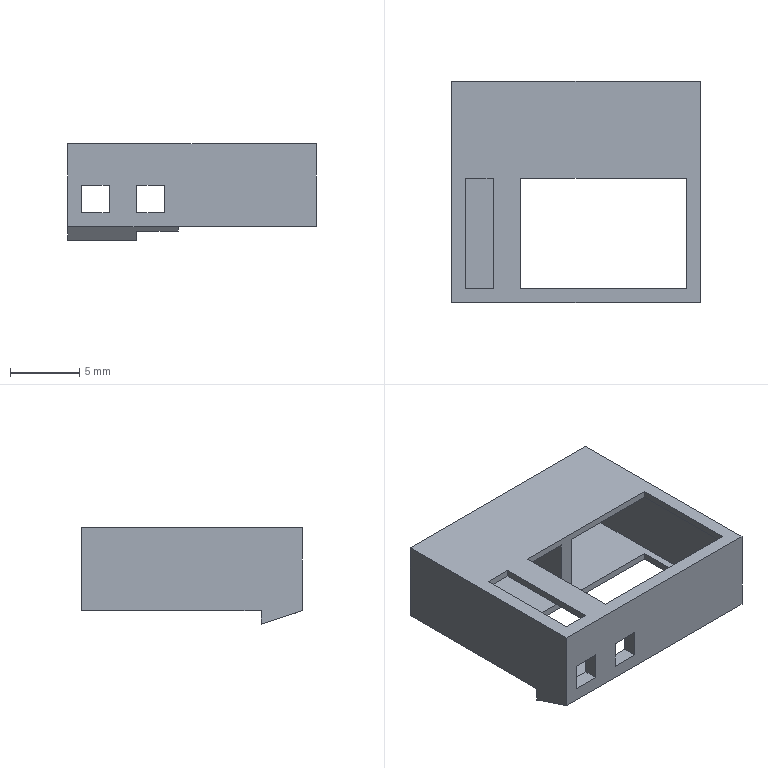Part | STEP file | 102000006983 | 1 solid | 34 faces | box 18 x 16 x 7 mm | volume 384 mm3 | plane 34
STEP:
#1=CARTESIAN_POINT('',(-9.,0.,0.));
#2=VERTEX_POINT('',#1);
#3=CARTESIAN_POINT('',(-9.,-13.,0.));
#4=VERTEX_POINT('',#3);
#5=CARTESIAN_POINT('',(-9.,-6.5,0.));
#6=DIRECTION('',(0.,-1.,0.));
#7=VECTOR('',#6,1.);
#8=LINE('',#5,#7);
#9=EDGE_CURVE('',#2,#4,#8,.T.);
#10=ORIENTED_EDGE('',*,*,#9,.T.);
#11=CARTESIAN_POINT('',(-9.,-13.,-1.));
#12=VERTEX_POINT('',#11);
#13=CARTESIAN_POINT('',(-9.,-13.,-0.5));
#14=DIRECTION('',(0.,0.,-1.));
#15=VECTOR('',#14,1.);
#16=LINE('',#13,#15);
#17=EDGE_CURVE('',#4,#12,#16,.T.);
#18=ORIENTED_EDGE('',*,*,#17,.T.);
#19=CARTESIAN_POINT('',(-9.,-16.,0.));
#20=VERTEX_POINT('',#19);
#21=CARTESIAN_POINT('',(-9.,-14.5,-0.5));
#22=DIRECTION('',(0.,-0.9487,0.3162));
#23=VECTOR('',#22,1.);
#24=LINE('',#21,#23);
#25=EDGE_CURVE('',#12,#20,#24,.T.);
#26=ORIENTED_EDGE('',*,*,#25,.T.);
#27=CARTESIAN_POINT('',(-9.,-16.,6.));
#28=VERTEX_POINT('',#27);
#29=CARTESIAN_POINT('',(-9.,-16.,3.));
#30=DIRECTION('',(0.,0.,-1.));
#31=VECTOR('',#30,1.);
#32=LINE('',#29,#31);
#33=EDGE_CURVE('',#28,#20,#32,.T.);
#34=ORIENTED_EDGE('',*,*,#33,.F.);
#35=CARTESIAN_POINT('',(-9.,0.,6.));
#36=VERTEX_POINT('',#35);
#37=CARTESIAN_POINT('',(-9.,-8.,6.));
#38=DIRECTION('',(0.,-1.,0.));
#39=VECTOR('',#38,1.);
#40=LINE('',#37,#39);
#41=EDGE_CURVE('',#36,#28,#40,.T.);
#42=ORIENTED_EDGE('',*,*,#41,.F.);
#43=CARTESIAN_POINT('',(-9.,0.,3.));
#44=DIRECTION('',(0.,0.,-1.));
#45=VECTOR('',#44,1.);
#46=LINE('',#43,#45);
#47=EDGE_CURVE('',#36,#2,#46,.T.);
#48=ORIENTED_EDGE('',*,*,#47,.T.);
#49=EDGE_LOOP('',(#10,#18,#26,#34,#42,#48));
#50=FACE_OUTER_BOUND('',#49,.T.);
#51=CARTESIAN_POINT('',(-9.,0.,6.));
#52=DIRECTION('',(1.,0.,0.));
#53=DIRECTION('',(0.,1.,0.));
#54=AXIS2_PLACEMENT_3D('',#51,#52,#53);
#55=PLANE('',#54);
#56=ADVANCED_FACE('',(#50),#55,.F.);
#57=CARTESIAN_POINT('',(-4.,-7.,0.));
#58=VERTEX_POINT('',#57);
#59=CARTESIAN_POINT('',(8.,-7.,0.));
#60=VERTEX_POINT('',#59);
#61=CARTESIAN_POINT('',(2.,-7.,0.));
#62=DIRECTION('',(1.,0.,0.));
#63=VECTOR('',#62,1.);
#64=LINE('',#61,#63);
#65=EDGE_CURVE('',#58,#60,#64,.T.);
#66=ORIENTED_EDGE('',*,*,#65,.F.);
#67=CARTESIAN_POINT('',(-4.,-13.,0.));
#68=VERTEX_POINT('',#67);
#69=CARTESIAN_POINT('',(-4.,-10.,0.));
#70=DIRECTION('',(0.,1.,0.));
#71=VECTOR('',#70,1.);
#72=LINE('',#69,#71);
#73=EDGE_CURVE('',#68,#58,#72,.T.);
#74=ORIENTED_EDGE('',*,*,#73,.F.);
#75=CARTESIAN_POINT('',(-6.5,-13.,0.));
#76=DIRECTION('',(-1.,0.,0.));
#77=VECTOR('',#76,1.);
#78=LINE('',#75,#77);
#79=EDGE_CURVE('',#68,#4,#78,.T.);
#80=ORIENTED_EDGE('',*,*,#79,.T.);
#81=ORIENTED_EDGE('',*,*,#9,.F.);
#82=CARTESIAN_POINT('',(9.,0.,0.));
#83=VERTEX_POINT('',#82);
#84=CARTESIAN_POINT('',(0.,0.,0.));
#85=DIRECTION('',(-1.,0.,0.));
#86=VECTOR('',#85,1.);
#87=LINE('',#84,#86);
#88=EDGE_CURVE('',#83,#2,#87,.T.);
#89=ORIENTED_EDGE('',*,*,#88,.F.);
#90=CARTESIAN_POINT('',(9.,-16.,0.));
#91=VERTEX_POINT('',#90);
#92=CARTESIAN_POINT('',(9.,-8.,0.));
#93=DIRECTION('',(0.,1.,0.));
#94=VECTOR('',#93,1.);
#95=LINE('',#92,#94);
#96=EDGE_CURVE('',#91,#83,#95,.T.);
#97=ORIENTED_EDGE('',*,*,#96,.F.);
#98=CARTESIAN_POINT('',(-1.,-16.,0.));
#99=VERTEX_POINT('',#98);
#100=CARTESIAN_POINT('',(4.,-16.,0.));
#101=DIRECTION('',(1.,0.,0.));
#102=VECTOR('',#101,1.);
#103=LINE('',#100,#102);
#104=EDGE_CURVE('',#99,#91,#103,.T.);
#105=ORIENTED_EDGE('',*,*,#104,.F.);
#106=CARTESIAN_POINT('',(-1.,-15.,0.));
#107=VERTEX_POINT('',#106);
#108=CARTESIAN_POINT('',(-1.,-15.5,0.));
#109=DIRECTION('',(0.,1.,0.));
#110=VECTOR('',#109,1.);
#111=LINE('',#108,#110);
#112=EDGE_CURVE('',#99,#107,#111,.T.);
#113=ORIENTED_EDGE('',*,*,#112,.T.);
#114=CARTESIAN_POINT('',(8.,-15.,0.));
#115=VERTEX_POINT('',#114);
#116=CARTESIAN_POINT('',(3.5,-15.,0.));
#117=DIRECTION('',(-1.,0.,0.));
#118=VECTOR('',#117,1.);
#119=LINE('',#116,#118);
#120=EDGE_CURVE('',#115,#107,#119,.T.);
#121=ORIENTED_EDGE('',*,*,#120,.F.);
#122=CARTESIAN_POINT('',(8.,-11.,0.));
#123=DIRECTION('',(0.,-1.,0.));
#124=VECTOR('',#123,1.);
#125=LINE('',#122,#124);
#126=EDGE_CURVE('',#60,#115,#125,.T.);
#127=ORIENTED_EDGE('',*,*,#126,.F.);
#128=EDGE_LOOP('',(#66,#74,#80,#81,#89,#97,#105,#113,#121,#127));
#129=FACE_OUTER_BOUND('',#128,.T.);
#130=CARTESIAN_POINT('',(0.,0.,0.));
#131=DIRECTION('',(0.,0.,1.));
#132=DIRECTION('',(1.,0.,0.));
#133=AXIS2_PLACEMENT_3D('',#130,#131,#132);
#134=PLANE('',#133);
#135=ADVANCED_FACE('',(#129),#134,.F.);
#136=CARTESIAN_POINT('',(-4.,-13.,-1.));
#137=VERTEX_POINT('',#136);
#138=CARTESIAN_POINT('',(-4.,-13.,-0.5));
#139=DIRECTION('',(0.,0.,-1.));
#140=VECTOR('',#139,1.);
#141=LINE('',#138,#140);
#142=EDGE_CURVE('',#68,#137,#141,.T.);
#143=ORIENTED_EDGE('',*,*,#142,.T.);
#144=CARTESIAN_POINT('',(-6.5,-13.,-1.));
#145=DIRECTION('',(-1.,0.,0.));
#146=VECTOR('',#145,1.);
#147=LINE('',#144,#146);
#148=EDGE_CURVE('',#137,#12,#147,.T.);
#149=ORIENTED_EDGE('',*,*,#148,.T.);
#150=ORIENTED_EDGE('',*,*,#17,.F.);
#151=ORIENTED_EDGE('',*,*,#79,.F.);
#152=EDGE_LOOP('',(#143,#149,#150,#151));
#153=FACE_OUTER_BOUND('',#152,.T.);
#154=CARTESIAN_POINT('',(-1.,-13.,-1.));
#155=DIRECTION('',(0.,1.,0.));
#156=DIRECTION('',(-1.,0.,0.));
#157=AXIS2_PLACEMENT_3D('',#154,#155,#156);
#158=PLANE('',#157);
#159=ADVANCED_FACE('',(#153),#158,.T.);
#160=CARTESIAN_POINT('',(-4.,-15.,-0.3333));
#161=VERTEX_POINT('',#160);
#162=CARTESIAN_POINT('',(-4.,-14.,-0.6667));
#163=DIRECTION('',(0.,-0.9487,0.3162));
#164=VECTOR('',#163,1.);
#165=LINE('',#162,#164);
#166=EDGE_CURVE('',#137,#161,#165,.T.);
#167=ORIENTED_EDGE('',*,*,#166,.T.);
#168=CARTESIAN_POINT('',(-1.,-15.,-0.3333));
#169=VERTEX_POINT('',#168);
#170=CARTESIAN_POINT('',(-2.5,-15.,-0.3333));
#171=DIRECTION('',(1.,0.,0.));
#172=VECTOR('',#171,1.);
#173=LINE('',#170,#172);
#174=EDGE_CURVE('',#161,#169,#173,.T.);
#175=ORIENTED_EDGE('',*,*,#174,.T.);
#176=CARTESIAN_POINT('',(-1.,-15.5,-0.1667));
#177=DIRECTION('',(0.,-0.9487,0.3162));
#178=VECTOR('',#177,1.);
#179=LINE('',#176,#178);
#180=EDGE_CURVE('',#169,#99,#179,.T.);
#181=ORIENTED_EDGE('',*,*,#180,.T.);
#182=CARTESIAN_POINT('',(-5.,-16.,0.));
#183=DIRECTION('',(1.,0.,0.));
#184=VECTOR('',#183,1.);
#185=LINE('',#182,#184);
#186=EDGE_CURVE('',#20,#99,#185,.T.);
#187=ORIENTED_EDGE('',*,*,#186,.F.);
#188=ORIENTED_EDGE('',*,*,#25,.F.);
#189=ORIENTED_EDGE('',*,*,#148,.F.);
#190=EDGE_LOOP('',(#167,#175,#181,#187,#188,#189));
#191=FACE_OUTER_BOUND('',#190,.T.);
#192=CARTESIAN_POINT('',(-1.,-16.,0.));
#193=DIRECTION('',(0.,-0.3162,-0.9487));
#194=DIRECTION('',(0.,0.9487,-0.3162));
#195=AXIS2_PLACEMENT_3D('',#192,#193,#194);
#196=PLANE('',#195);
#197=ADVANCED_FACE('',(#191),#196,.T.);
#198=ORIENTED_EDGE('',*,*,#186,.T.);
#199=ORIENTED_EDGE('',*,*,#104,.T.);
#200=CARTESIAN_POINT('',(9.,-16.,6.));
#201=VERTEX_POINT('',#200);
#202=CARTESIAN_POINT('',(9.,-16.,3.));
#203=DIRECTION('',(0.,0.,-1.));
#204=VECTOR('',#203,1.);
#205=LINE('',#202,#204);
#206=EDGE_CURVE('',#201,#91,#205,.T.);
#207=ORIENTED_EDGE('',*,*,#206,.F.);
#208=CARTESIAN_POINT('',(0.,-16.,6.));
#209=DIRECTION('',(1.,0.,0.));
#210=VECTOR('',#209,1.);
#211=LINE('',#208,#210);
#212=EDGE_CURVE('',#28,#201,#211,.T.);
#213=ORIENTED_EDGE('',*,*,#212,.F.);
#214=ORIENTED_EDGE('',*,*,#33,.T.);
#215=EDGE_LOOP('',(#198,#199,#207,#213,#214));
#216=FACE_OUTER_BOUND('',#215,.T.);
#217=CARTESIAN_POINT('',(-4.,-16.,1.));
#218=VERTEX_POINT('',#217);
#219=CARTESIAN_POINT('',(-2.,-16.,1.));
#220=VERTEX_POINT('',#219);
#221=CARTESIAN_POINT('',(-3.,-16.,1.));
#222=DIRECTION('',(1.,0.,0.));
#223=VECTOR('',#222,1.);
#224=LINE('',#221,#223);
#225=EDGE_CURVE('',#218,#220,#224,.T.);
#226=ORIENTED_EDGE('',*,*,#225,.F.);
#227=CARTESIAN_POINT('',(-4.,-16.,3.));
#228=VERTEX_POINT('',#227);
#229=CARTESIAN_POINT('',(-4.,-16.,2.));
#230=DIRECTION('',(0.,0.,-1.));
#231=VECTOR('',#230,1.);
#232=LINE('',#229,#231);
#233=EDGE_CURVE('',#228,#218,#232,.T.);
#234=ORIENTED_EDGE('',*,*,#233,.F.);
#235=CARTESIAN_POINT('',(-2.,-16.,3.));
#236=VERTEX_POINT('',#235);
#237=CARTESIAN_POINT('',(-3.,-16.,3.));
#238=DIRECTION('',(-1.,0.,0.));
#239=VECTOR('',#238,1.);
#240=LINE('',#237,#239);
#241=EDGE_CURVE('',#236,#228,#240,.T.);
#242=ORIENTED_EDGE('',*,*,#241,.F.);
#243=CARTESIAN_POINT('',(-2.,-16.,2.));
#244=DIRECTION('',(0.,0.,1.));
#245=VECTOR('',#244,1.);
#246=LINE('',#243,#245);
#247=EDGE_CURVE('',#220,#236,#246,.T.);
#248=ORIENTED_EDGE('',*,*,#247,.F.);
#249=EDGE_LOOP('',(#226,#234,#242,#248));
#250=FACE_BOUND('',#249,.T.);
#251=CARTESIAN_POINT('',(-8.,-16.,1.));
#252=VERTEX_POINT('',#251);
#253=CARTESIAN_POINT('',(-6.,-16.,1.));
#254=VERTEX_POINT('',#253);
#255=CARTESIAN_POINT('',(-7.,-16.,1.));
#256=DIRECTION('',(1.,0.,0.));
#257=VECTOR('',#256,1.);
#258=LINE('',#255,#257);
#259=EDGE_CURVE('',#252,#254,#258,.T.);
#260=ORIENTED_EDGE('',*,*,#259,.F.);
#261=CARTESIAN_POINT('',(-8.,-16.,3.));
#262=VERTEX_POINT('',#261);
#263=CARTESIAN_POINT('',(-8.,-16.,2.));
#264=DIRECTION('',(0.,0.,-1.));
#265=VECTOR('',#264,1.);
#266=LINE('',#263,#265);
#267=EDGE_CURVE('',#262,#252,#266,.T.);
#268=ORIENTED_EDGE('',*,*,#267,.F.);
#269=CARTESIAN_POINT('',(-6.,-16.,3.));
#270=VERTEX_POINT('',#269);
#271=CARTESIAN_POINT('',(-7.,-16.,3.));
#272=DIRECTION('',(-1.,0.,0.));
#273=VECTOR('',#272,1.);
#274=LINE('',#271,#273);
#275=EDGE_CURVE('',#270,#262,#274,.T.);
#276=ORIENTED_EDGE('',*,*,#275,.F.);
#277=CARTESIAN_POINT('',(-6.,-16.,2.));
#278=DIRECTION('',(0.,0.,1.));
#279=VECTOR('',#278,1.);
#280=LINE('',#277,#279);
#281=EDGE_CURVE('',#254,#270,#280,.T.);
#282=ORIENTED_EDGE('',*,*,#281,.F.);
#283=EDGE_LOOP('',(#260,#268,#276,#282));
#284=FACE_BOUND('',#283,.T.);
#285=CARTESIAN_POINT('',(-9.,-16.,6.));
#286=DIRECTION('',(0.,1.,0.));
#287=DIRECTION('',(0.,0.,1.));
#288=AXIS2_PLACEMENT_3D('',#285,#286,#287);
#289=PLANE('',#288);
#290=ADVANCED_FACE('',(#216,#250,#284),#289,.F.);
#291=ORIENTED_EDGE('',*,*,#41,.T.);
#292=ORIENTED_EDGE('',*,*,#212,.T.);
#293=CARTESIAN_POINT('',(9.,0.,6.));
#294=VERTEX_POINT('',#293);
#295=CARTESIAN_POINT('',(9.,-8.,6.));
#296=DIRECTION('',(0.,1.,0.));
#297=VECTOR('',#296,1.);
#298=LINE('',#295,#297);
#299=EDGE_CURVE('',#201,#294,#298,.T.);
#300=ORIENTED_EDGE('',*,*,#299,.T.);
#301=CARTESIAN_POINT('',(0.,0.,6.));
#302=DIRECTION('',(-1.,0.,0.));
#303=VECTOR('',#302,1.);
#304=LINE('',#301,#303);
#305=EDGE_CURVE('',#294,#36,#304,.T.);
#306=ORIENTED_EDGE('',*,*,#305,.T.);
#307=EDGE_LOOP('',(#291,#292,#300,#306));
#308=FACE_OUTER_BOUND('',#307,.T.);
#309=CARTESIAN_POINT('',(-4.,-7.,6.));
#310=VERTEX_POINT('',#309);
#311=CARTESIAN_POINT('',(-4.,-15.,6.));
#312=VERTEX_POINT('',#311);
#313=CARTESIAN_POINT('',(-4.,-11.,6.));
#314=DIRECTION('',(0.,-1.,0.));
#315=VECTOR('',#314,1.);
#316=LINE('',#313,#315);
#317=EDGE_CURVE('',#310,#312,#316,.T.);
#318=ORIENTED_EDGE('',*,*,#317,.F.);
#319=CARTESIAN_POINT('',(8.,-7.,6.));
#320=VERTEX_POINT('',#319);
#321=CARTESIAN_POINT('',(2.,-7.,6.));
#322=DIRECTION('',(-1.,0.,0.));
#323=VECTOR('',#322,1.);
#324=LINE('',#321,#323);
#325=EDGE_CURVE('',#320,#310,#324,.T.);
#326=ORIENTED_EDGE('',*,*,#325,.F.);
#327=CARTESIAN_POINT('',(8.,-15.,6.));
#328=VERTEX_POINT('',#327);
#329=CARTESIAN_POINT('',(8.,-11.,6.));
#330=DIRECTION('',(0.,1.,0.));
#331=VECTOR('',#330,1.);
#332=LINE('',#329,#331);
#333=EDGE_CURVE('',#328,#320,#332,.T.);
#334=ORIENTED_EDGE('',*,*,#333,.F.);
#335=CARTESIAN_POINT('',(2.,-15.,6.));
#336=DIRECTION('',(1.,0.,0.));
#337=VECTOR('',#336,1.);
#338=LINE('',#335,#337);
#339=EDGE_CURVE('',#312,#328,#338,.T.);
#340=ORIENTED_EDGE('',*,*,#339,.F.);
#341=EDGE_LOOP('',(#318,#326,#334,#340));
#342=FACE_BOUND('',#341,.T.);
#343=CARTESIAN_POINT('',(-8.,-7.,6.));
#344=VERTEX_POINT('',#343);
#345=CARTESIAN_POINT('',(-8.,-15.,6.));
#346=VERTEX_POINT('',#345);
#347=CARTESIAN_POINT('',(-8.,-11.,6.));
#348=DIRECTION('',(0.,-1.,0.));
#349=VECTOR('',#348,1.);
#350=LINE('',#347,#349);
#351=EDGE_CURVE('',#344,#346,#350,.T.);
#352=ORIENTED_EDGE('',*,*,#351,.F.);
#353=CARTESIAN_POINT('',(-6.,-7.,6.));
#354=VERTEX_POINT('',#353);
#355=CARTESIAN_POINT('',(-7.,-7.,6.));
#356=DIRECTION('',(-1.,0.,0.));
#357=VECTOR('',#356,1.);
#358=LINE('',#355,#357);
#359=EDGE_CURVE('',#354,#344,#358,.T.);
#360=ORIENTED_EDGE('',*,*,#359,.F.);
#361=CARTESIAN_POINT('',(-6.,-15.,6.));
#362=VERTEX_POINT('',#361);
#363=CARTESIAN_POINT('',(-6.,-11.,6.));
#364=DIRECTION('',(0.,1.,0.));
#365=VECTOR('',#364,1.);
#366=LINE('',#363,#365);
#367=EDGE_CURVE('',#362,#354,#366,.T.);
#368=ORIENTED_EDGE('',*,*,#367,.F.);
#369=CARTESIAN_POINT('',(-7.,-15.,6.));
#370=DIRECTION('',(1.,0.,0.));
#371=VECTOR('',#370,1.);
#372=LINE('',#369,#371);
#373=EDGE_CURVE('',#346,#362,#372,.T.);
#374=ORIENTED_EDGE('',*,*,#373,.F.);
#375=EDGE_LOOP('',(#352,#360,#368,#374));
#376=FACE_BOUND('',#375,.T.);
#377=CARTESIAN_POINT('',(0.,0.,6.));
#378=DIRECTION('',(0.,0.,1.));
#379=DIRECTION('',(1.,0.,0.));
#380=AXIS2_PLACEMENT_3D('',#377,#378,#379);
#381=PLANE('',#380);
#382=ADVANCED_FACE('',(#308,#342,#376),#381,.T.);
#383=ORIENTED_EDGE('',*,*,#88,.T.);
#384=ORIENTED_EDGE('',*,*,#47,.F.);
#385=ORIENTED_EDGE('',*,*,#305,.F.);
#386=CARTESIAN_POINT('',(9.,0.,3.));
#387=DIRECTION('',(0.,0.,-1.));
#388=VECTOR('',#387,1.);
#389=LINE('',#386,#388);
#390=EDGE_CURVE('',#294,#83,#389,.T.);
#391=ORIENTED_EDGE('',*,*,#390,.T.);
#392=EDGE_LOOP('',(#383,#384,#385,#391));
#393=FACE_OUTER_BOUND('',#392,.T.);
#394=CARTESIAN_POINT('',(0.5,0.,5.5));
#395=VERTEX_POINT('',#394);
#396=CARTESIAN_POINT('',(8.5,0.,5.5));
#397=VERTEX_POINT('',#396);
#398=CARTESIAN_POINT('',(4.5,0.,5.5));
#399=DIRECTION('',(1.,0.,0.));
#400=VECTOR('',#399,1.);
#401=LINE('',#398,#400);
#402=EDGE_CURVE('',#395,#397,#401,.T.);
#403=ORIENTED_EDGE('',*,*,#402,.F.);
#404=CARTESIAN_POINT('',(0.5,0.,0.5));
#405=VERTEX_POINT('',#404);
#406=CARTESIAN_POINT('',(0.5,0.,3.));
#407=DIRECTION('',(0.,0.,1.));
#408=VECTOR('',#407,1.);
#409=LINE('',#406,#408);
#410=EDGE_CURVE('',#405,#395,#409,.T.);
#411=ORIENTED_EDGE('',*,*,#410,.F.);
#412=CARTESIAN_POINT('',(8.5,0.,0.5));
#413=VERTEX_POINT('',#412);
#414=CARTESIAN_POINT('',(4.5,0.,0.5));
#415=DIRECTION('',(-1.,0.,0.));
#416=VECTOR('',#415,1.);
#417=LINE('',#414,#416);
#418=EDGE_CURVE('',#413,#405,#417,.T.);
#419=ORIENTED_EDGE('',*,*,#418,.F.);
#420=CARTESIAN_POINT('',(8.5,0.,3.));
#421=DIRECTION('',(0.,0.,-1.));
#422=VECTOR('',#421,1.);
#423=LINE('',#420,#422);
#424=EDGE_CURVE('',#397,#413,#423,.T.);
#425=ORIENTED_EDGE('',*,*,#424,.F.);
#426=EDGE_LOOP('',(#403,#411,#419,#425));
#427=FACE_BOUND('',#426,.T.);
#428=CARTESIAN_POINT('',(-8.5,0.,5.5));
#429=VERTEX_POINT('',#428);
#430=CARTESIAN_POINT('',(-0.5,0.,5.5));
#431=VERTEX_POINT('',#430);
#432=CARTESIAN_POINT('',(-4.5,0.,5.5));
#433=DIRECTION('',(1.,0.,0.));
#434=VECTOR('',#433,1.);
#435=LINE('',#432,#434);
#436=EDGE_CURVE('',#429,#431,#435,.T.);
#437=ORIENTED_EDGE('',*,*,#436,.F.);
#438=CARTESIAN_POINT('',(-8.5,0.,0.5));
#439=VERTEX_POINT('',#438);
#440=CARTESIAN_POINT('',(-8.5,0.,3.));
#441=DIRECTION('',(0.,0.,1.));
#442=VECTOR('',#441,1.);
#443=LINE('',#440,#442);
#444=EDGE_CURVE('',#439,#429,#443,.T.);
#445=ORIENTED_EDGE('',*,*,#444,.F.);
#446=CARTESIAN_POINT('',(-0.5,0.,0.5));
#447=VERTEX_POINT('',#446);
#448=CARTESIAN_POINT('',(-4.5,0.,0.5));
#449=DIRECTION('',(-1.,0.,0.));
#450=VECTOR('',#449,1.);
#451=LINE('',#448,#450);
#452=EDGE_CURVE('',#447,#439,#451,.T.);
#453=ORIENTED_EDGE('',*,*,#452,.F.);
#454=CARTESIAN_POINT('',(-0.5,0.,3.));
#455=DIRECTION('',(0.,0.,-1.));
#456=VECTOR('',#455,1.);
#457=LINE('',#454,#456);
#458=EDGE_CURVE('',#431,#447,#457,.T.);
#459=ORIENTED_EDGE('',*,*,#458,.F.);
#460=EDGE_LOOP('',(#437,#445,#453,#459));
#461=FACE_BOUND('',#460,.T.);
#462=CARTESIAN_POINT('',(-9.,0.,6.));
#463=DIRECTION('',(0.,-1.,0.));
#464=DIRECTION('',(0.,0.,-1.));
#465=AXIS2_PLACEMENT_3D('',#462,#463,#464);
#466=PLANE('',#465);
#467=ADVANCED_FACE('',(#393,#427,#461),#466,.F.);
#468=ORIENTED_EDGE('',*,*,#65,.T.);
#469=CARTESIAN_POINT('',(8.,-7.,0.5));
#470=VERTEX_POINT('',#469);
#471=CARTESIAN_POINT('',(8.,-7.,0.25));
#472=DIRECTION('',(0.,0.,1.));
#473=VECTOR('',#472,1.);
#474=LINE('',#471,#473);
#475=EDGE_CURVE('',#60,#470,#474,.T.);
#476=ORIENTED_EDGE('',*,*,#475,.T.);
#477=CARTESIAN_POINT('',(0.5,-7.,0.5));
#478=VERTEX_POINT('',#477);
#479=CARTESIAN_POINT('',(4.25,-7.,0.5));
#480=DIRECTION('',(-1.,0.,0.));
#481=VECTOR('',#480,1.);
#482=LINE('',#479,#481);
#483=EDGE_CURVE('',#470,#478,#482,.T.);
#484=ORIENTED_EDGE('',*,*,#483,.T.);
#485=CARTESIAN_POINT('',(0.5,-7.,5.5));
#486=VERTEX_POINT('',#485);
#487=CARTESIAN_POINT('',(0.5,-7.,3.));
#488=DIRECTION('',(0.,0.,1.));
#489=VECTOR('',#488,1.);
#490=LINE('',#487,#489);
#491=EDGE_CURVE('',#478,#486,#490,.T.);
#492=ORIENTED_EDGE('',*,*,#491,.T.);
#493=CARTESIAN_POINT('',(8.,-7.,5.5));
#494=VERTEX_POINT('',#493);
#495=CARTESIAN_POINT('',(4.25,-7.,5.5));
#496=DIRECTION('',(1.,0.,0.));
#497=VECTOR('',#496,1.);
#498=LINE('',#495,#497);
#499=EDGE_CURVE('',#486,#494,#498,.T.);
#500=ORIENTED_EDGE('',*,*,#499,.T.);
#501=CARTESIAN_POINT('',(8.,-7.,5.75));
#502=DIRECTION('',(0.,0.,1.));
#503=VECTOR('',#502,1.);
#504=LINE('',#501,#503);
#505=EDGE_CURVE('',#494,#320,#504,.T.);
#506=ORIENTED_EDGE('',*,*,#505,.T.);
#507=ORIENTED_EDGE('',*,*,#325,.T.);
#508=CARTESIAN_POINT('',(-4.,-7.,5.5));
#509=VERTEX_POINT('',#508);
#510=CARTESIAN_POINT('',(-4.,-7.,5.75));
#511=DIRECTION('',(0.,0.,1.));
#512=VECTOR('',#511,1.);
#513=LINE('',#510,#512);
#514=EDGE_CURVE('',#509,#310,#513,.T.);
#515=ORIENTED_EDGE('',*,*,#514,.F.);
#516=CARTESIAN_POINT('',(-0.5,-7.,5.5));
#517=VERTEX_POINT('',#516);
#518=CARTESIAN_POINT('',(-2.25,-7.,5.5));
#519=DIRECTION('',(1.,0.,0.));
#520=VECTOR('',#519,1.);
#521=LINE('',#518,#520);
#522=EDGE_CURVE('',#509,#517,#521,.T.);
#523=ORIENTED_EDGE('',*,*,#522,.T.);
#524=CARTESIAN_POINT('',(-0.5,-7.,0.5));
#525=VERTEX_POINT('',#524);
#526=CARTESIAN_POINT('',(-0.5,-7.,3.));
#527=DIRECTION('',(0.,0.,-1.));
#528=VECTOR('',#527,1.);
#529=LINE('',#526,#528);
#530=EDGE_CURVE('',#517,#525,#529,.T.);
#531=ORIENTED_EDGE('',*,*,#530,.T.);
#532=CARTESIAN_POINT('',(-4.,-7.,0.5));
#533=VERTEX_POINT('',#532);
#534=CARTESIAN_POINT('',(-2.25,-7.,0.5));
#535=DIRECTION('',(-1.,0.,0.));
#536=VECTOR('',#535,1.);
#537=LINE('',#534,#536);
#538=EDGE_CURVE('',#525,#533,#537,.T.);
#539=ORIENTED_EDGE('',*,*,#538,.T.);
#540=CARTESIAN_POINT('',(-4.,-7.,0.25));
#541=DIRECTION('',(0.,0.,1.));
#542=VECTOR('',#541,1.);
#543=LINE('',#540,#542);
#544=EDGE_CURVE('',#58,#533,#543,.T.);
#545=ORIENTED_EDGE('',*,*,#544,.F.);
#546=EDGE_LOOP('',(#468,#476,#484,#492,#500,#506,#507,#515,#523,#531,#539,#545));
#547=FACE_OUTER_BOUND('',#546,.T.);
#548=CARTESIAN_POINT('',(-4.,-7.,-1.001));
#549=DIRECTION('',(0.,1.,0.));
#550=DIRECTION('',(0.,0.,1.));
#551=AXIS2_PLACEMENT_3D('',#548,#549,#550);
#552=PLANE('',#551);
#553=ADVANCED_FACE('',(#547),#552,.F.);
#554=CARTESIAN_POINT('',(-4.,-15.,0.5));
#555=VERTEX_POINT('',#554);
#556=CARTESIAN_POINT('',(-4.,-11.,0.5));
#557=DIRECTION('',(0.,-1.,0.));
#558=VECTOR('',#557,1.);
#559=LINE('',#556,#558);
#560=EDGE_CURVE('',#533,#555,#559,.T.);
#561=ORIENTED_EDGE('',*,*,#560,.T.);
#562=CARTESIAN_POINT('',(-4.,-15.,0.08333));
#563=DIRECTION('',(0.,0.,1.));
#564=VECTOR('',#563,1.);
#565=LINE('',#562,#564);
#566=EDGE_CURVE('',#161,#555,#565,.T.);
#567=ORIENTED_EDGE('',*,*,#566,.F.);
#568=ORIENTED_EDGE('',*,*,#166,.F.);
#569=ORIENTED_EDGE('',*,*,#142,.F.);
#570=ORIENTED_EDGE('',*,*,#73,.T.);
#571=ORIENTED_EDGE('',*,*,#544,.T.);
#572=EDGE_LOOP('',(#561,#567,#568,#569,#570,#571));
#573=FACE_OUTER_BOUND('',#572,.T.);
#574=CARTESIAN_POINT('',(-4.,-7.,-1.001));
#575=DIRECTION('',(-1.,0.,0.));
#576=DIRECTION('',(0.,-1.,0.));
#577=AXIS2_PLACEMENT_3D('',#574,#575,#576);
#578=PLANE('',#577);
#579=ADVANCED_FACE('',(#573),#578,.F.);
#580=ORIENTED_EDGE('',*,*,#96,.T.);
#581=ORIENTED_EDGE('',*,*,#390,.F.);
#582=ORIENTED_EDGE('',*,*,#299,.F.);
#583=ORIENTED_EDGE('',*,*,#206,.T.);
#584=EDGE_LOOP('',(#580,#581,#582,#583));
#585=FACE_OUTER_BOUND('',#584,.T.);
#586=CARTESIAN_POINT('',(9.,0.,6.));
#587=DIRECTION('',(-1.,0.,0.));
#588=DIRECTION('',(0.,-1.,0.));
#589=AXIS2_PLACEMENT_3D('',#586,#587,#588);
#590=PLANE('',#589);
#591=ADVANCED_FACE('',(#585),#590,.F.);
#592=CARTESIAN_POINT('',(-1.,-15.,-0.1667));
#593=DIRECTION('',(0.,0.,1.));
#594=VECTOR('',#593,1.);
#595=LINE('',#592,#594);
#596=EDGE_CURVE('',#169,#107,#595,.T.);
#597=ORIENTED_EDGE('',*,*,#596,.T.);
#598=ORIENTED_EDGE('',*,*,#112,.F.);
#599=ORIENTED_EDGE('',*,*,#180,.F.);
#600=EDGE_LOOP('',(#597,#598,#599));
#601=FACE_OUTER_BOUND('',#600,.T.);
#602=CARTESIAN_POINT('',(-1.,0.,0.));
#603=DIRECTION('',(1.,0.,0.));
#604=DIRECTION('',(0.,0.,-1.));
#605=AXIS2_PLACEMENT_3D('',#602,#603,#604);
#606=PLANE('',#605);
#607=ADVANCED_FACE('',(#601),#606,.T.);
#608=ORIENTED_EDGE('',*,*,#566,.T.);
#609=CARTESIAN_POINT('',(-8.5,-15.,0.5));
#610=VERTEX_POINT('',#609);
#611=CARTESIAN_POINT('',(-6.25,-15.,0.5));
#612=DIRECTION('',(-1.,0.,0.));
#613=VECTOR('',#612,1.);
#614=LINE('',#611,#613);
#615=EDGE_CURVE('',#555,#610,#614,.T.);
#616=ORIENTED_EDGE('',*,*,#615,.T.);
#617=CARTESIAN_POINT('',(-8.5,-15.,5.5));
#618=VERTEX_POINT('',#617);
#619=CARTESIAN_POINT('',(-8.5,-15.,3.));
#620=DIRECTION('',(0.,0.,1.));
#621=VECTOR('',#620,1.);
#622=LINE('',#619,#621);
#623=EDGE_CURVE('',#610,#618,#622,.T.);
#624=ORIENTED_EDGE('',*,*,#623,.T.);
#625=CARTESIAN_POINT('',(-8.,-15.,5.5));
#626=VERTEX_POINT('',#625);
#627=CARTESIAN_POINT('',(-8.25,-15.,5.5));
#628=DIRECTION('',(1.,0.,0.));
#629=VECTOR('',#628,1.);
#630=LINE('',#627,#629);
#631=EDGE_CURVE('',#618,#626,#630,.T.);
#632=ORIENTED_EDGE('',*,*,#631,.T.);
#633=CARTESIAN_POINT('',(-8.,-15.,5.75));
#634=DIRECTION('',(0.,0.,1.));
#635=VECTOR('',#634,1.);
#636=LINE('',#633,#635);
#637=EDGE_CURVE('',#626,#346,#636,.T.);
#638=ORIENTED_EDGE('',*,*,#637,.T.);
#639=ORIENTED_EDGE('',*,*,#373,.T.);
#640=CARTESIAN_POINT('',(-6.,-15.,5.5));
#641=VERTEX_POINT('',#640);
#642=CARTESIAN_POINT('',(-6.,-15.,5.75));
#643=DIRECTION('',(0.,0.,1.));
#644=VECTOR('',#643,1.);
#645=LINE('',#642,#644);
#646=EDGE_CURVE('',#641,#362,#645,.T.);
#647=ORIENTED_EDGE('',*,*,#646,.F.);
#648=CARTESIAN_POINT('',(-4.,-15.,5.5));
#649=VERTEX_POINT('',#648);
#650=CARTESIAN_POINT('',(-5.,-15.,5.5));
#651=DIRECTION('',(1.,0.,0.));
#652=VECTOR('',#651,1.);
#653=LINE('',#650,#652);
#654=EDGE_CURVE('',#641,#649,#653,.T.);
#655=ORIENTED_EDGE('',*,*,#654,.T.);
#656=CARTESIAN_POINT('',(-4.,-15.,5.75));
#657=DIRECTION('',(0.,0.,1.));
#658=VECTOR('',#657,1.);
#659=LINE('',#656,#658);
#660=EDGE_CURVE('',#649,#312,#659,.T.);
#661=ORIENTED_EDGE('',*,*,#660,.T.);
#662=ORIENTED_EDGE('',*,*,#339,.T.);
#663=CARTESIAN_POINT('',(8.,-15.,5.5));
#664=VERTEX_POINT('',#663);
#665=CARTESIAN_POINT('',(8.,-15.,5.75));
#666=DIRECTION('',(0.,0.,1.));
#667=VECTOR('',#666,1.);
#668=LINE('',#665,#667);
#669=EDGE_CURVE('',#664,#328,#668,.T.);
#670=ORIENTED_EDGE('',*,*,#669,.F.);
#671=CARTESIAN_POINT('',(8.5,-15.,5.5));
#672=VERTEX_POINT('',#671);
#673=CARTESIAN_POINT('',(8.25,-15.,5.5));
#674=DIRECTION('',(1.,0.,0.));
#675=VECTOR('',#674,1.);
#676=LINE('',#673,#675);
#677=EDGE_CURVE('',#664,#672,#676,.T.);
#678=ORIENTED_EDGE('',*,*,#677,.T.);
#679=CARTESIAN_POINT('',(8.5,-15.,0.5));
#680=VERTEX_POINT('',#679);
#681=CARTESIAN_POINT('',(8.5,-15.,3.));
#682=DIRECTION('',(0.,0.,-1.));
#683=VECTOR('',#682,1.);
#684=LINE('',#681,#683);
#685=EDGE_CURVE('',#672,#680,#684,.T.);
#686=ORIENTED_EDGE('',*,*,#685,.T.);
#687=CARTESIAN_POINT('',(8.,-15.,0.5));
#688=VERTEX_POINT('',#687);
#689=CARTESIAN_POINT('',(8.25,-15.,0.5));
#690=DIRECTION('',(-1.,0.,0.));
#691=VECTOR('',#690,1.);
#692=LINE('',#689,#691);
#693=EDGE_CURVE('',#680,#688,#692,.T.);
#694=ORIENTED_EDGE('',*,*,#693,.T.);
#695=CARTESIAN_POINT('',(8.,-15.,0.25));
#696=DIRECTION('',(0.,0.,1.));
#697=VECTOR('',#696,1.);
#698=LINE('',#695,#697);
#699=EDGE_CURVE('',#115,#688,#698,.T.);
#700=ORIENTED_EDGE('',*,*,#699,.F.);
#701=ORIENTED_EDGE('',*,*,#120,.T.);
#702=ORIENTED_EDGE('',*,*,#596,.F.);
#703=ORIENTED_EDGE('',*,*,#174,.F.);
#704=EDGE_LOOP('',(#608,#616,#624,#632,#638,#639,#647,#655,#661,#662,#670,#678,#686,#694,#700,#701,#702,#703));
#705=FACE_OUTER_BOUND('',#704,.T.);
#706=CARTESIAN_POINT('',(-4.,-15.,1.));
#707=VERTEX_POINT('',#706);
#708=CARTESIAN_POINT('',(-4.,-15.,3.));
#709=VERTEX_POINT('',#708);
#710=CARTESIAN_POINT('',(-4.,-15.,2.));
#711=DIRECTION('',(0.,0.,1.));
#712=VECTOR('',#711,1.);
#713=LINE('',#710,#712);
#714=EDGE_CURVE('',#707,#709,#713,.T.);
#715=ORIENTED_EDGE('',*,*,#714,.F.);
#716=CARTESIAN_POINT('',(-2.,-15.,1.));
#717=VERTEX_POINT('',#716);
#718=CARTESIAN_POINT('',(-3.,-15.,1.));
#719=DIRECTION('',(-1.,0.,0.));
#720=VECTOR('',#719,1.);
#721=LINE('',#718,#720);
#722=EDGE_CURVE('',#717,#707,#721,.T.);
#723=ORIENTED_EDGE('',*,*,#722,.F.);
#724=CARTESIAN_POINT('',(-2.,-15.,3.));
#725=VERTEX_POINT('',#724);
#726=CARTESIAN_POINT('',(-2.,-15.,2.));
#727=DIRECTION('',(0.,0.,-1.));
#728=VECTOR('',#727,1.);
#729=LINE('',#726,#728);
#730=EDGE_CURVE('',#725,#717,#729,.T.);
#731=ORIENTED_EDGE('',*,*,#730,.F.);
#732=CARTESIAN_POINT('',(-3.,-15.,3.));
#733=DIRECTION('',(1.,0.,0.));
#734=VECTOR('',#733,1.);
#735=LINE('',#732,#734);
#736=EDGE_CURVE('',#709,#725,#735,.T.);
#737=ORIENTED_EDGE('',*,*,#736,.F.);
#738=EDGE_LOOP('',(#715,#723,#731,#737));
#739=FACE_BOUND('',#738,.T.);
#740=CARTESIAN_POINT('',(-8.,-15.,1.));
#741=VERTEX_POINT('',#740);
#742=CARTESIAN_POINT('',(-8.,-15.,3.));
#743=VERTEX_POINT('',#742);
#744=CARTESIAN_POINT('',(-8.,-15.,2.));
#745=DIRECTION('',(0.,0.,1.));
#746=VECTOR('',#745,1.);
#747=LINE('',#744,#746);
#748=EDGE_CURVE('',#741,#743,#747,.T.);
#749=ORIENTED_EDGE('',*,*,#748,.F.);
#750=CARTESIAN_POINT('',(-6.,-15.,1.));
#751=VERTEX_POINT('',#750);
#752=CARTESIAN_POINT('',(-7.,-15.,1.));
#753=DIRECTION('',(-1.,0.,0.));
#754=VECTOR('',#753,1.);
#755=LINE('',#752,#754);
#756=EDGE_CURVE('',#751,#741,#755,.T.);
#757=ORIENTED_EDGE('',*,*,#756,.F.);
#758=CARTESIAN_POINT('',(-6.,-15.,3.));
#759=VERTEX_POINT('',#758);
#760=CARTESIAN_POINT('',(-6.,-15.,2.));
#761=DIRECTION('',(0.,0.,-1.));
#762=VECTOR('',#761,1.);
#763=LINE('',#760,#762);
#764=EDGE_CURVE('',#759,#751,#763,.T.);
#765=ORIENTED_EDGE('',*,*,#764,.F.);
#766=CARTESIAN_POINT('',(-7.,-15.,3.));
#767=DIRECTION('',(1.,0.,0.));
#768=VECTOR('',#767,1.);
#769=LINE('',#766,#768);
#770=EDGE_CURVE('',#743,#759,#769,.T.);
#771=ORIENTED_EDGE('',*,*,#770,.F.);
#772=EDGE_LOOP('',(#749,#757,#765,#771));
#773=FACE_BOUND('',#772,.T.);
#774=CARTESIAN_POINT('',(0.,-15.,0.));
#775=DIRECTION('',(0.,1.,0.));
#776=DIRECTION('',(0.,0.,1.));
#777=AXIS2_PLACEMENT_3D('',#774,#775,#776);
#778=PLANE('',#777);
#779=ADVANCED_FACE('',(#705,#739,#773),#778,.T.);
#780=ORIENTED_EDGE('',*,*,#126,.T.);
#781=ORIENTED_EDGE('',*,*,#699,.T.);
#782=CARTESIAN_POINT('',(8.,-11.,0.5));
#783=DIRECTION('',(0.,1.,0.));
#784=VECTOR('',#783,1.);
#785=LINE('',#782,#784);
#786=EDGE_CURVE('',#688,#470,#785,.T.);
#787=ORIENTED_EDGE('',*,*,#786,.T.);
#788=ORIENTED_EDGE('',*,*,#475,.F.);
#789=EDGE_LOOP('',(#780,#781,#787,#788));
#790=FACE_OUTER_BOUND('',#789,.T.);
#791=CARTESIAN_POINT('',(8.,-7.,-1.001));
#792=DIRECTION('',(1.,0.,0.));
#793=DIRECTION('',(0.,0.,-1.));
#794=AXIS2_PLACEMENT_3D('',#791,#792,#793);
#795=PLANE('',#794);
#796=ADVANCED_FACE('',(#790),#795,.F.);
#797=ORIENTED_EDGE('',*,*,#722,.T.);
#798=CARTESIAN_POINT('',(-4.,-15.5,1.));
#799=DIRECTION('',(0.,-1.,0.));
#800=VECTOR('',#799,1.);
#801=LINE('',#798,#800);
#802=EDGE_CURVE('',#707,#218,#801,.T.);
#803=ORIENTED_EDGE('',*,*,#802,.T.);
#804=ORIENTED_EDGE('',*,*,#225,.T.);
#805=CARTESIAN_POINT('',(-2.,-15.5,1.));
#806=DIRECTION('',(0.,-1.,0.));
#807=VECTOR('',#806,1.);
#808=LINE('',#805,#807);
#809=EDGE_CURVE('',#717,#220,#808,.T.);
#810=ORIENTED_EDGE('',*,*,#809,.F.);
#811=EDGE_LOOP('',(#797,#803,#804,#810));
#812=FACE_OUTER_BOUND('',#811,.T.);
#813=CARTESIAN_POINT('',(-4.,0.,1.));
#814=DIRECTION('',(0.,0.,-1.));
#815=DIRECTION('',(-1.,0.,0.));
#816=AXIS2_PLACEMENT_3D('',#813,#814,#815);
#817=PLANE('',#816);
#818=ADVANCED_FACE('',(#812),#817,.F.);
#819=ORIENTED_EDGE('',*,*,#714,.T.);
#820=CARTESIAN_POINT('',(-4.,-15.5,3.));
#821=DIRECTION('',(0.,-1.,0.));
#822=VECTOR('',#821,1.);
#823=LINE('',#820,#822);
#824=EDGE_CURVE('',#709,#228,#823,.T.);
#825=ORIENTED_EDGE('',*,*,#824,.T.);
#826=ORIENTED_EDGE('',*,*,#233,.T.);
#827=ORIENTED_EDGE('',*,*,#802,.F.);
#828=EDGE_LOOP('',(#819,#825,#826,#827));
#829=FACE_OUTER_BOUND('',#828,.T.);
#830=CARTESIAN_POINT('',(-4.,0.,3.));
#831=DIRECTION('',(-1.,0.,0.));
#832=DIRECTION('',(0.,0.,1.));
#833=AXIS2_PLACEMENT_3D('',#830,#831,#832);
#834=PLANE('',#833);
#835=ADVANCED_FACE('',(#829),#834,.F.);
#836=ORIENTED_EDGE('',*,*,#736,.T.);
#837=CARTESIAN_POINT('',(-2.,-15.5,3.));
#838=DIRECTION('',(0.,-1.,0.));
#839=VECTOR('',#838,1.);
#840=LINE('',#837,#839);
#841=EDGE_CURVE('',#725,#236,#840,.T.);
#842=ORIENTED_EDGE('',*,*,#841,.T.);
#843=ORIENTED_EDGE('',*,*,#241,.T.);
#844=ORIENTED_EDGE('',*,*,#824,.F.);
#845=EDGE_LOOP('',(#836,#842,#843,#844));
#846=FACE_OUTER_BOUND('',#845,.T.);
#847=CARTESIAN_POINT('',(-4.,0.,3.));
#848=DIRECTION('',(0.,0.,1.));
#849=DIRECTION('',(1.,0.,0.));
#850=AXIS2_PLACEMENT_3D('',#847,#848,#849);
#851=PLANE('',#850);
#852=ADVANCED_FACE('',(#846),#851,.F.);
#853=ORIENTED_EDGE('',*,*,#730,.T.);
#854=ORIENTED_EDGE('',*,*,#809,.T.);
#855=ORIENTED_EDGE('',*,*,#247,.T.);
#856=ORIENTED_EDGE('',*,*,#841,.F.);
#857=EDGE_LOOP('',(#853,#854,#855,#856));
#858=FACE_OUTER_BOUND('',#857,.T.);
#859=CARTESIAN_POINT('',(-2.,0.,3.));
#860=DIRECTION('',(1.,0.,0.));
#861=DIRECTION('',(0.,0.,-1.));
#862=AXIS2_PLACEMENT_3D('',#859,#860,#861);
#863=PLANE('',#862);
#864=ADVANCED_FACE('',(#858),#863,.F.);
#865=ORIENTED_EDGE('',*,*,#756,.T.);
#866=CARTESIAN_POINT('',(-8.,-15.5,1.));
#867=DIRECTION('',(0.,-1.,0.));
#868=VECTOR('',#867,1.);
#869=LINE('',#866,#868);
#870=EDGE_CURVE('',#741,#252,#869,.T.);
#871=ORIENTED_EDGE('',*,*,#870,.T.);
#872=ORIENTED_EDGE('',*,*,#259,.T.);
#873=CARTESIAN_POINT('',(-6.,-15.5,1.));
#874=DIRECTION('',(0.,-1.,0.));
#875=VECTOR('',#874,1.);
#876=LINE('',#873,#875);
#877=EDGE_CURVE('',#751,#254,#876,.T.);
#878=ORIENTED_EDGE('',*,*,#877,.F.);
#879=EDGE_LOOP('',(#865,#871,#872,#878));
#880=FACE_OUTER_BOUND('',#879,.T.);
#881=CARTESIAN_POINT('',(-8.,0.,1.));
#882=DIRECTION('',(0.,0.,-1.));
#883=DIRECTION('',(-1.,0.,0.));
#884=AXIS2_PLACEMENT_3D('',#881,#882,#883);
#885=PLANE('',#884);
#886=ADVANCED_FACE('',(#880),#885,.F.);
#887=ORIENTED_EDGE('',*,*,#748,.T.);
#888=CARTESIAN_POINT('',(-8.,-15.5,3.));
#889=DIRECTION('',(0.,-1.,0.));
#890=VECTOR('',#889,1.);
#891=LINE('',#888,#890);
#892=EDGE_CURVE('',#743,#262,#891,.T.);
#893=ORIENTED_EDGE('',*,*,#892,.T.);
#894=ORIENTED_EDGE('',*,*,#267,.T.);
#895=ORIENTED_EDGE('',*,*,#870,.F.);
#896=EDGE_LOOP('',(#887,#893,#894,#895));
#897=FACE_OUTER_BOUND('',#896,.T.);
#898=CARTESIAN_POINT('',(-8.,0.,3.));
#899=DIRECTION('',(-1.,0.,0.));
#900=DIRECTION('',(0.,0.,1.));
#901=AXIS2_PLACEMENT_3D('',#898,#899,#900);
#902=PLANE('',#901);
#903=ADVANCED_FACE('',(#897),#902,.F.);
#904=ORIENTED_EDGE('',*,*,#770,.T.);
#905=CARTESIAN_POINT('',(-6.,-15.5,3.));
#906=DIRECTION('',(0.,-1.,0.));
#907=VECTOR('',#906,1.);
#908=LINE('',#905,#907);
#909=EDGE_CURVE('',#759,#270,#908,.T.);
#910=ORIENTED_EDGE('',*,*,#909,.T.);
#911=ORIENTED_EDGE('',*,*,#275,.T.);
#912=ORIENTED_EDGE('',*,*,#892,.F.);
#913=EDGE_LOOP('',(#904,#910,#911,#912));
#914=FACE_OUTER_BOUND('',#913,.T.);
#915=CARTESIAN_POINT('',(-8.,0.,3.));
#916=DIRECTION('',(0.,0.,1.));
#917=DIRECTION('',(1.,0.,0.));
#918=AXIS2_PLACEMENT_3D('',#915,#916,#917);
#919=PLANE('',#918);
#920=ADVANCED_FACE('',(#914),#919,.F.);
#921=ORIENTED_EDGE('',*,*,#764,.T.);
#922=ORIENTED_EDGE('',*,*,#877,.T.);
#923=ORIENTED_EDGE('',*,*,#281,.T.);
#924=ORIENTED_EDGE('',*,*,#909,.F.);
#925=EDGE_LOOP('',(#921,#922,#923,#924));
#926=FACE_OUTER_BOUND('',#925,.T.);
#927=CARTESIAN_POINT('',(-6.,0.,3.));
#928=DIRECTION('',(1.,0.,0.));
#929=DIRECTION('',(0.,0.,-1.));
#930=AXIS2_PLACEMENT_3D('',#927,#928,#929);
#931=PLANE('',#930);
#932=ADVANCED_FACE('',(#926),#931,.F.);
#933=CARTESIAN_POINT('',(-4.,-11.,5.5));
#934=DIRECTION('',(0.,1.,0.));
#935=VECTOR('',#934,1.);
#936=LINE('',#933,#935);
#937=EDGE_CURVE('',#649,#509,#936,.T.);
#938=ORIENTED_EDGE('',*,*,#937,.T.);
#939=ORIENTED_EDGE('',*,*,#514,.T.);
#940=ORIENTED_EDGE('',*,*,#317,.T.);
#941=ORIENTED_EDGE('',*,*,#660,.F.);
#942=EDGE_LOOP('',(#938,#939,#940,#941));
#943=FACE_OUTER_BOUND('',#942,.T.);
#944=CARTESIAN_POINT('',(-4.,-7.,-1.001));
#945=DIRECTION('',(-1.,0.,0.));
#946=DIRECTION('',(0.,-1.,0.));
#947=AXIS2_PLACEMENT_3D('',#944,#945,#946);
#948=PLANE('',#947);
#949=ADVANCED_FACE('',(#943),#948,.F.);
#950=CARTESIAN_POINT('',(8.,-11.,5.5));
#951=DIRECTION('',(0.,-1.,0.));
#952=VECTOR('',#951,1.);
#953=LINE('',#950,#952);
#954=EDGE_CURVE('',#494,#664,#953,.T.);
#955=ORIENTED_EDGE('',*,*,#954,.T.);
#956=ORIENTED_EDGE('',*,*,#669,.T.);
#957=ORIENTED_EDGE('',*,*,#333,.T.);
#958=ORIENTED_EDGE('',*,*,#505,.F.);
#959=EDGE_LOOP('',(#955,#956,#957,#958));
#960=FACE_OUTER_BOUND('',#959,.T.);
#961=CARTESIAN_POINT('',(8.,-7.,-1.001));
#962=DIRECTION('',(1.,0.,0.));
#963=DIRECTION('',(0.,0.,-1.));
#964=AXIS2_PLACEMENT_3D('',#961,#962,#963);
#965=PLANE('',#964);
#966=ADVANCED_FACE('',(#960),#965,.F.);
#967=CARTESIAN_POINT('',(-8.,-7.,5.5));
#968=VERTEX_POINT('',#967);
#969=CARTESIAN_POINT('',(-8.,-11.,5.5));
#970=DIRECTION('',(0.,1.,0.));
#971=VECTOR('',#970,1.);
#972=LINE('',#969,#971);
#973=EDGE_CURVE('',#626,#968,#972,.T.);
#974=ORIENTED_EDGE('',*,*,#973,.T.);
#975=CARTESIAN_POINT('',(-8.,-7.,5.75));
#976=DIRECTION('',(0.,0.,1.));
#977=VECTOR('',#976,1.);
#978=LINE('',#975,#977);
#979=EDGE_CURVE('',#968,#344,#978,.T.);
#980=ORIENTED_EDGE('',*,*,#979,.T.);
#981=ORIENTED_EDGE('',*,*,#351,.T.);
#982=ORIENTED_EDGE('',*,*,#637,.F.);
#983=EDGE_LOOP('',(#974,#980,#981,#982));
#984=FACE_OUTER_BOUND('',#983,.T.);
#985=CARTESIAN_POINT('',(-8.,-7.,-1.001));
#986=DIRECTION('',(-1.,0.,0.));
#987=DIRECTION('',(0.,-1.,0.));
#988=AXIS2_PLACEMENT_3D('',#985,#986,#987);
#989=PLANE('',#988);
#990=ADVANCED_FACE('',(#984),#989,.F.);
#991=CARTESIAN_POINT('',(-6.,-7.,5.5));
#992=VERTEX_POINT('',#991);
#993=CARTESIAN_POINT('',(-7.,-7.,5.5));
#994=DIRECTION('',(1.,0.,0.));
#995=VECTOR('',#994,1.);
#996=LINE('',#993,#995);
#997=EDGE_CURVE('',#968,#992,#996,.T.);
#998=ORIENTED_EDGE('',*,*,#997,.T.);
#999=CARTESIAN_POINT('',(-6.,-7.,5.75));
#1000=DIRECTION('',(0.,0.,1.));
#1001=VECTOR('',#1000,1.);
#1002=LINE('',#999,#1001);
#1003=EDGE_CURVE('',#992,#354,#1002,.T.);
#1004=ORIENTED_EDGE('',*,*,#1003,.T.);
#1005=ORIENTED_EDGE('',*,*,#359,.T.);
#1006=ORIENTED_EDGE('',*,*,#979,.F.);
#1007=EDGE_LOOP('',(#998,#1004,#1005,#1006));
#1008=FACE_OUTER_BOUND('',#1007,.T.);
#1009=CARTESIAN_POINT('',(-8.,-7.,-1.001));
#1010=DIRECTION('',(0.,1.,0.));
#1011=DIRECTION('',(0.,0.,1.));
#1012=AXIS2_PLACEMENT_3D('',#1009,#1010,#1011);
#1013=PLANE('',#1012);
#1014=ADVANCED_FACE('',(#1008),#1013,.F.);
#1015=CARTESIAN_POINT('',(-6.,-11.,5.5));
#1016=DIRECTION('',(0.,-1.,0.));
#1017=VECTOR('',#1016,1.);
#1018=LINE('',#1015,#1017);
#1019=EDGE_CURVE('',#992,#641,#1018,.T.);
#1020=ORIENTED_EDGE('',*,*,#1019,.T.);
#1021=ORIENTED_EDGE('',*,*,#646,.T.);
#1022=ORIENTED_EDGE('',*,*,#367,.T.);
#1023=ORIENTED_EDGE('',*,*,#1003,.F.);
#1024=EDGE_LOOP('',(#1020,#1021,#1022,#1023));
#1025=FACE_OUTER_BOUND('',#1024,.T.);
#1026=CARTESIAN_POINT('',(-6.,-7.,-1.001));
#1027=DIRECTION('',(1.,0.,0.));
#1028=DIRECTION('',(0.,1.,0.));
#1029=AXIS2_PLACEMENT_3D('',#1026,#1027,#1028);
#1030=PLANE('',#1029);
#1031=ADVANCED_FACE('',(#1025),#1030,.F.);
#1032=ORIENTED_EDGE('',*,*,#954,.F.);
#1033=ORIENTED_EDGE('',*,*,#499,.F.);
#1034=CARTESIAN_POINT('',(0.5,-3.5,5.5));
#1035=DIRECTION('',(0.,1.,0.));
#1036=VECTOR('',#1035,1.);
#1037=LINE('',#1034,#1036);
#1038=EDGE_CURVE('',#486,#395,#1037,.T.);
#1039=ORIENTED_EDGE('',*,*,#1038,.T.);
#1040=ORIENTED_EDGE('',*,*,#402,.T.);
#1041=CARTESIAN_POINT('',(8.5,-7.5,5.5));
#1042=DIRECTION('',(0.,1.,0.));
#1043=VECTOR('',#1042,1.);
#1044=LINE('',#1041,#1043);
#1045=EDGE_CURVE('',#672,#397,#1044,.T.);
#1046=ORIENTED_EDGE('',*,*,#1045,.F.);
#1047=ORIENTED_EDGE('',*,*,#677,.F.);
#1048=EDGE_LOOP('',(#1032,#1033,#1039,#1040,#1046,#1047));
#1049=FACE_OUTER_BOUND('',#1048,.T.);
#1050=CARTESIAN_POINT('',(0.5,-15.,5.5));
#1051=DIRECTION('',(0.,0.,1.));
#1052=DIRECTION('',(1.,0.,0.));
#1053=AXIS2_PLACEMENT_3D('',#1050,#1051,#1052);
#1054=PLANE('',#1053);
#1055=ADVANCED_FACE('',(#1049),#1054,.F.);
#1056=ORIENTED_EDGE('',*,*,#1038,.F.);
#1057=ORIENTED_EDGE('',*,*,#491,.F.);
#1058=CARTESIAN_POINT('',(0.5,-3.5,0.5));
#1059=DIRECTION('',(0.,1.,0.));
#1060=VECTOR('',#1059,1.);
#1061=LINE('',#1058,#1060);
#1062=EDGE_CURVE('',#478,#405,#1061,.T.);
#1063=ORIENTED_EDGE('',*,*,#1062,.T.);
#1064=ORIENTED_EDGE('',*,*,#410,.T.);
#1065=EDGE_LOOP('',(#1056,#1057,#1063,#1064));
#1066=FACE_OUTER_BOUND('',#1065,.T.);
#1067=CARTESIAN_POINT('',(0.5,-15.,0.5));
#1068=DIRECTION('',(-1.,0.,0.));
#1069=DIRECTION('',(0.,0.,1.));
#1070=AXIS2_PLACEMENT_3D('',#1067,#1068,#1069);
#1071=PLANE('',#1070);
#1072=ADVANCED_FACE('',(#1066),#1071,.F.);
#1073=ORIENTED_EDGE('',*,*,#1062,.F.);
#1074=ORIENTED_EDGE('',*,*,#483,.F.);
#1075=ORIENTED_EDGE('',*,*,#786,.F.);
#1076=ORIENTED_EDGE('',*,*,#693,.F.);
#1077=CARTESIAN_POINT('',(8.5,-7.5,0.5));
#1078=DIRECTION('',(0.,1.,0.));
#1079=VECTOR('',#1078,1.);
#1080=LINE('',#1077,#1079);
#1081=EDGE_CURVE('',#680,#413,#1080,.T.);
#1082=ORIENTED_EDGE('',*,*,#1081,.T.);
#1083=ORIENTED_EDGE('',*,*,#418,.T.);
#1084=EDGE_LOOP('',(#1073,#1074,#1075,#1076,#1082,#1083));
#1085=FACE_OUTER_BOUND('',#1084,.T.);
#1086=CARTESIAN_POINT('',(0.5,-15.,0.5));
#1087=DIRECTION('',(0.,0.,-1.));
#1088=DIRECTION('',(-1.,0.,0.));
#1089=AXIS2_PLACEMENT_3D('',#1086,#1087,#1088);
#1090=PLANE('',#1089);
#1091=ADVANCED_FACE('',(#1085),#1090,.F.);
#1092=ORIENTED_EDGE('',*,*,#424,.T.);
#1093=ORIENTED_EDGE('',*,*,#1081,.F.);
#1094=ORIENTED_EDGE('',*,*,#685,.F.);
#1095=ORIENTED_EDGE('',*,*,#1045,.T.);
#1096=EDGE_LOOP('',(#1092,#1093,#1094,#1095));
#1097=FACE_OUTER_BOUND('',#1096,.T.);
#1098=CARTESIAN_POINT('',(8.5,-15.,0.5));
#1099=DIRECTION('',(1.,0.,0.));
#1100=DIRECTION('',(0.,0.,-1.));
#1101=AXIS2_PLACEMENT_3D('',#1098,#1099,#1100);
#1102=PLANE('',#1101);
#1103=ADVANCED_FACE('',(#1097),#1102,.F.);
#1104=ORIENTED_EDGE('',*,*,#522,.F.);
#1105=ORIENTED_EDGE('',*,*,#937,.F.);
#1106=ORIENTED_EDGE('',*,*,#654,.F.);
#1107=ORIENTED_EDGE('',*,*,#1019,.F.);
#1108=ORIENTED_EDGE('',*,*,#997,.F.);
#1109=ORIENTED_EDGE('',*,*,#973,.F.);
#1110=ORIENTED_EDGE('',*,*,#631,.F.);
#1111=CARTESIAN_POINT('',(-8.5,-7.5,5.5));
#1112=DIRECTION('',(0.,1.,0.));
#1113=VECTOR('',#1112,1.);
#1114=LINE('',#1111,#1113);
#1115=EDGE_CURVE('',#618,#429,#1114,.T.);
#1116=ORIENTED_EDGE('',*,*,#1115,.T.);
#1117=ORIENTED_EDGE('',*,*,#436,.T.);
#1118=CARTESIAN_POINT('',(-0.5,-3.5,5.5));
#1119=DIRECTION('',(0.,1.,0.));
#1120=VECTOR('',#1119,1.);
#1121=LINE('',#1118,#1120);
#1122=EDGE_CURVE('',#517,#431,#1121,.T.);
#1123=ORIENTED_EDGE('',*,*,#1122,.F.);
#1124=EDGE_LOOP('',(#1104,#1105,#1106,#1107,#1108,#1109,#1110,#1116,#1117,#1123));
#1125=FACE_OUTER_BOUND('',#1124,.T.);
#1126=CARTESIAN_POINT('',(-8.5,-15.,5.5));
#1127=DIRECTION('',(0.,0.,1.));
#1128=DIRECTION('',(1.,0.,0.));
#1129=AXIS2_PLACEMENT_3D('',#1126,#1127,#1128);
#1130=PLANE('',#1129);
#1131=ADVANCED_FACE('',(#1125),#1130,.F.);
#1132=ORIENTED_EDGE('',*,*,#444,.T.);
#1133=ORIENTED_EDGE('',*,*,#1115,.F.);
#1134=ORIENTED_EDGE('',*,*,#623,.F.);
#1135=CARTESIAN_POINT('',(-8.5,-7.5,0.5));
#1136=DIRECTION('',(0.,1.,0.));
#1137=VECTOR('',#1136,1.);
#1138=LINE('',#1135,#1137);
#1139=EDGE_CURVE('',#610,#439,#1138,.T.);
#1140=ORIENTED_EDGE('',*,*,#1139,.T.);
#1141=EDGE_LOOP('',(#1132,#1133,#1134,#1140));
#1142=FACE_OUTER_BOUND('',#1141,.T.);
#1143=CARTESIAN_POINT('',(-8.5,-15.,0.5));
#1144=DIRECTION('',(-1.,0.,0.));
#1145=DIRECTION('',(0.,0.,1.));
#1146=AXIS2_PLACEMENT_3D('',#1143,#1144,#1145);
#1147=PLANE('',#1146);
#1148=ADVANCED_FACE('',(#1142),#1147,.F.);
#1149=ORIENTED_EDGE('',*,*,#615,.F.);
#1150=ORIENTED_EDGE('',*,*,#560,.F.);
#1151=ORIENTED_EDGE('',*,*,#538,.F.);
#1152=CARTESIAN_POINT('',(-0.5,-3.5,0.5));
#1153=DIRECTION('',(0.,1.,0.));
#1154=VECTOR('',#1153,1.);
#1155=LINE('',#1152,#1154);
#1156=EDGE_CURVE('',#525,#447,#1155,.T.);
#1157=ORIENTED_EDGE('',*,*,#1156,.T.);
#1158=ORIENTED_EDGE('',*,*,#452,.T.);
#1159=ORIENTED_EDGE('',*,*,#1139,.F.);
#1160=EDGE_LOOP('',(#1149,#1150,#1151,#1157,#1158,#1159));
#1161=FACE_OUTER_BOUND('',#1160,.T.);
#1162=CARTESIAN_POINT('',(-8.5,-15.,0.5));
#1163=DIRECTION('',(0.,0.,-1.));
#1164=DIRECTION('',(-1.,0.,0.));
#1165=AXIS2_PLACEMENT_3D('',#1162,#1163,#1164);
#1166=PLANE('',#1165);
#1167=ADVANCED_FACE('',(#1161),#1166,.F.);
#1168=ORIENTED_EDGE('',*,*,#1156,.F.);
#1169=ORIENTED_EDGE('',*,*,#530,.F.);
#1170=ORIENTED_EDGE('',*,*,#1122,.T.);
#1171=ORIENTED_EDGE('',*,*,#458,.T.);
#1172=EDGE_LOOP('',(#1168,#1169,#1170,#1171));
#1173=FACE_OUTER_BOUND('',#1172,.T.);
#1174=CARTESIAN_POINT('',(-0.5,-15.,0.5));
#1175=DIRECTION('',(1.,0.,0.));
#1176=DIRECTION('',(0.,0.,-1.));
#1177=AXIS2_PLACEMENT_3D('',#1174,#1175,#1176);
#1178=PLANE('',#1177);
#1179=ADVANCED_FACE('',(#1173),#1178,.F.);
#1180=CLOSED_SHELL('',(#56,#135,#159,#197,#290,#382,#467,#553,#579,#591,#607,#779,#796,#818,#835,#852,#864,#886,#903,#920,#932,#949,#966,#990,#1014,#1031,#1055,#1072,#1091,#1103,#1131,#1148,#1167,#1179));
#1181=MANIFOLD_SOLID_BREP('',#1180);
#1182=(LENGTH_UNIT()NAMED_UNIT(*)SI_UNIT(.MILLI.,.METRE.));
#1183=UNCERTAINTY_MEASURE_WITH_UNIT(LENGTH_MEASURE(0.005),#1182,'','');
#1184=(NAMED_UNIT(*)PLANE_ANGLE_UNIT()SI_UNIT($,.RADIAN.));
#1185=(NAMED_UNIT(*)SI_UNIT($,.STERADIAN.)SOLID_ANGLE_UNIT());
#1186=(GEOMETRIC_REPRESENTATION_CONTEXT(3)GLOBAL_UNCERTAINTY_ASSIGNED_CONTEXT((#1183))GLOBAL_UNIT_ASSIGNED_CONTEXT((#1182,#1184,#1185))REPRESENTATION_CONTEXT('',''));
#1187=ADVANCED_BREP_SHAPE_REPRESENTATION('',(#1181),#1186);